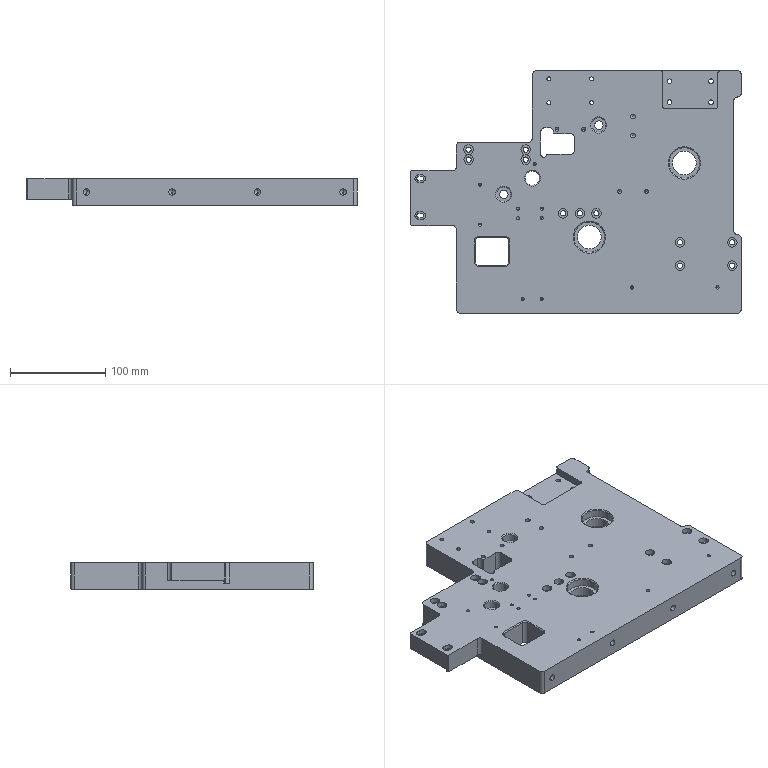Part | STEP file | 10000020440swp000-1 | 1 solid | 370 faces | box 348 x 255 x 28 mm | volume 1845671 mm3 | cylinder 201 | cone 86 | plane 83 | commonest cylinder face diameters 3.3 x38 8 x26 5.5 x22 10 x22 4 x16 4.2 x16